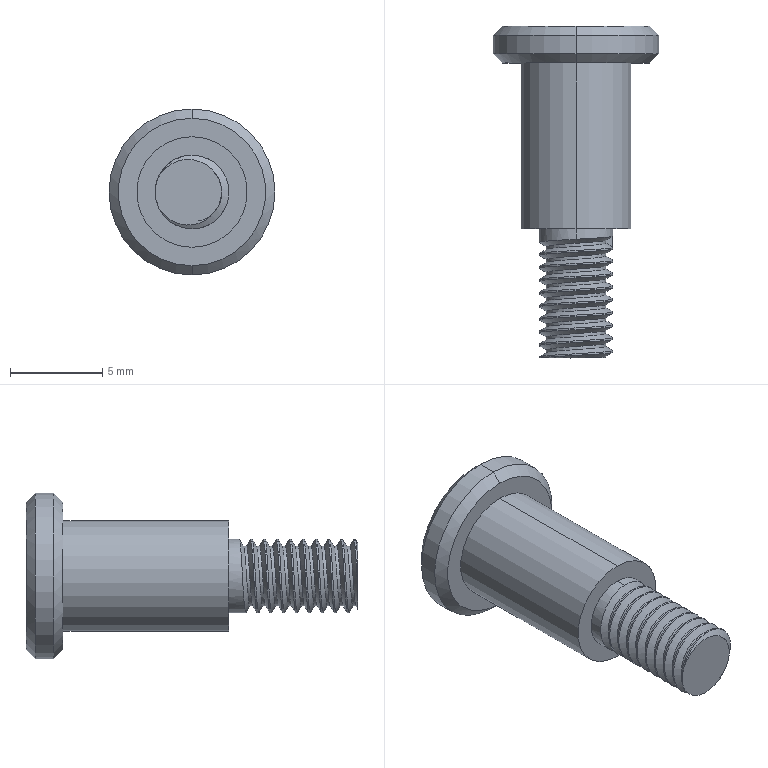Part | NX | features BREP 1 | 1 solid | 42 faces | box 9 x 18 x 9 mm | volume 417.74 mm3 | cylinder 24 | plane 12 | cone 4 | spline 2 | commonest cylinder face diameters 4 x19 6 x2 9 x2 3.242 x1